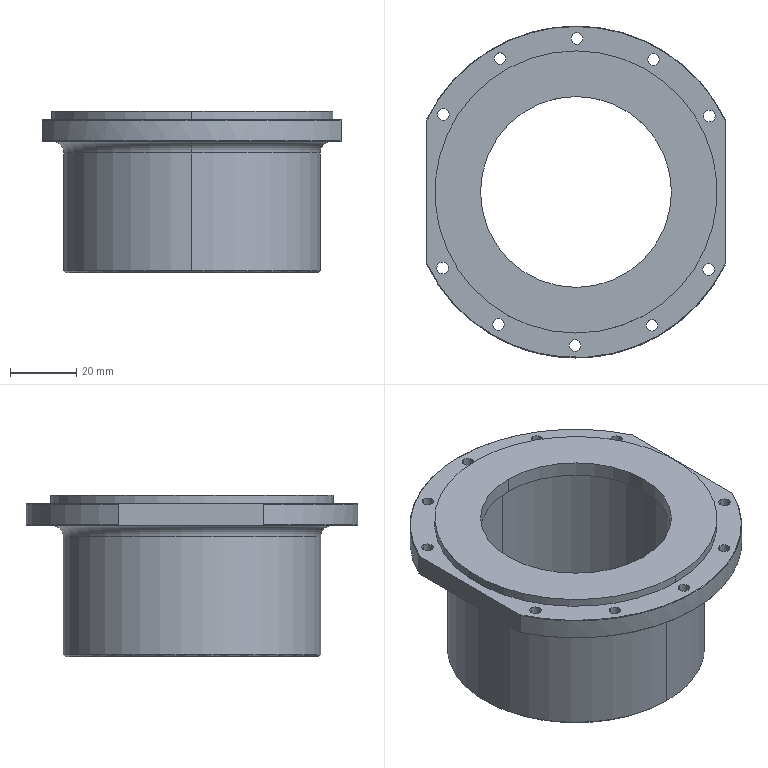Part | STEP file | 2026.6.15-Main Assembly图.sldasm-Part-148 | 1 solid | 72 faces | box 90.222 x 100 x 48.5 mm | volume 102684 mm3 | cylinder 47 | plane 15 | cone 8 | torus 2 | commonest cylinder face diameters 3.5 x20 2.5 x16 100 x3 57.5 x2 62.5 x2 77.5 x2